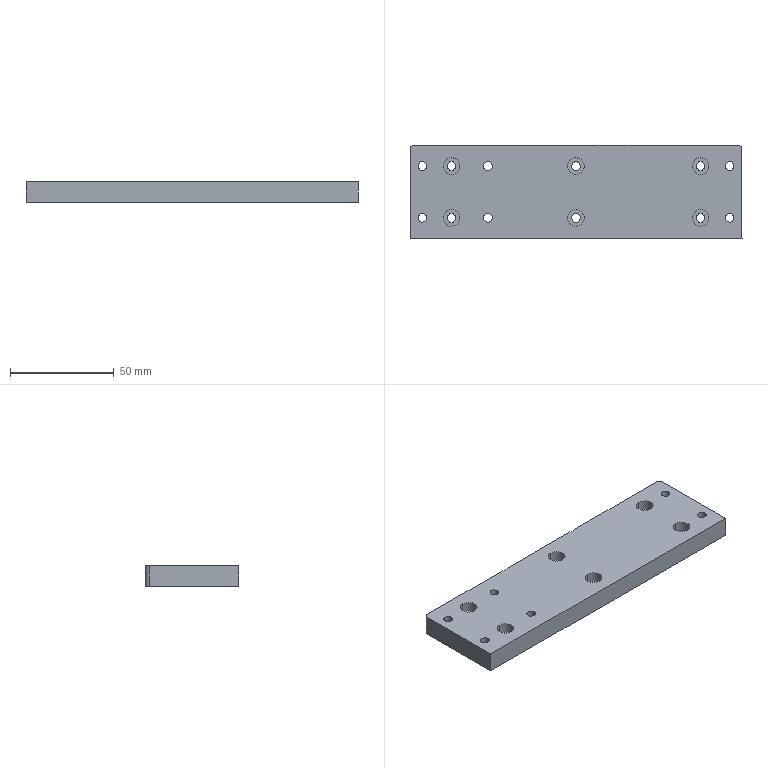Part | SolidWorks | features BaseBody 1 | 1 solid | 88 faces | box 160 x 45 x 10 mm | volume 67785 mm3 | cylinder 66 | plane 22 | commonest cylinder face diameters 8 x30 4.2 x24 3.3 x6 10 x4 4 x2